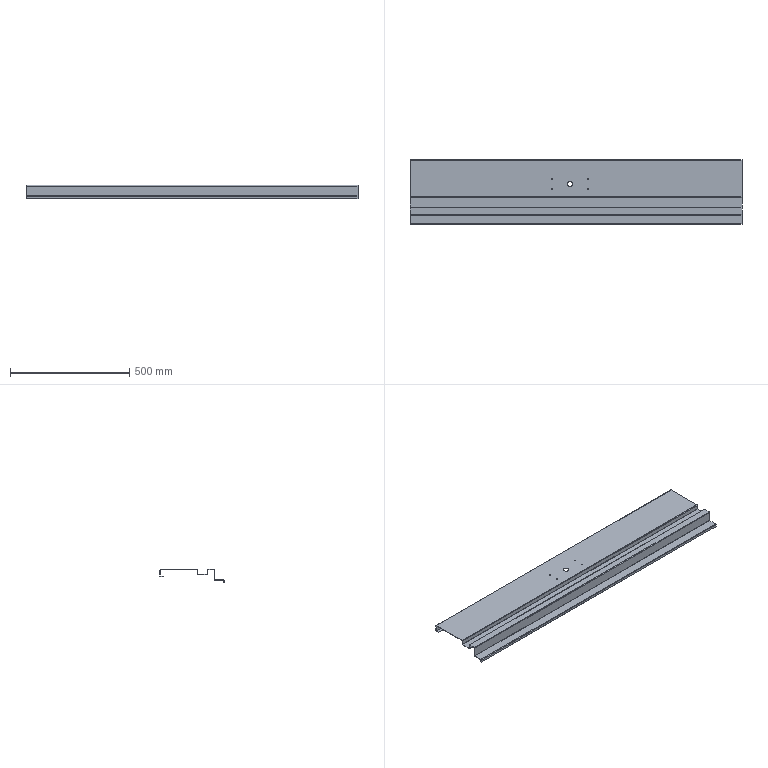Part | STEP file | Front Plate | 1 solid | 52 faces | box 1390 x 268 x 55 mm | volume 1100627 mm3 | cylinder 28 | plane 24 | commonest cylinder face diameters 1 x9 5 x9 3.2 x8 22 x2